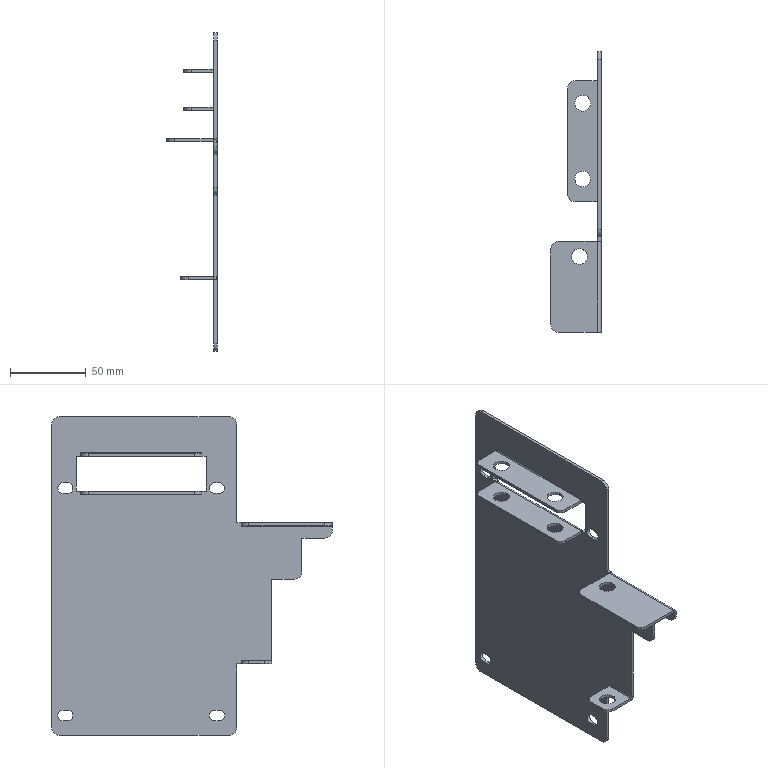Part | STEP file | 1 solid | 104 faces | box 33 x 185 x 210 mm | volume 62468 mm3 | plane 62 | cylinder 42 | commonest cylinder face diameters 10 x14 10.5 x12 7 x8 1 x4 5 x4